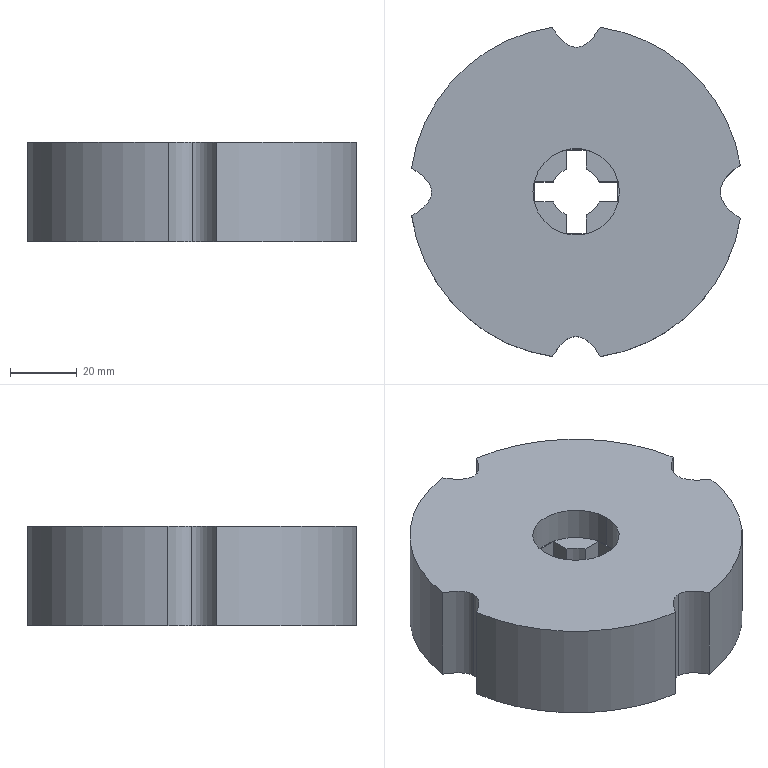Part | SolidWorks | features Extrusion 1, ICE 1 | 1 solid | 33 faces | box 98.826 x 98.952 x 30 mm | volume 216398 mm3 | plane 15 | cylinder 10 | spline 8 | commonest cylinder face diameters 15 x4 100 x4 26 x2
STEP:
#1=CARTESIAN_POINT('',(-13.,0.,5.));
#2=VERTEX_POINT('',#1);
#3=CARTESIAN_POINT('',(13.,0.,5.));
#4=VERTEX_POINT('',#3);
#5=CARTESIAN_POINT('',(0.,0.,5.));
#6=DIRECTION('',(0.,0.,1.));
#7=DIRECTION('',(1.,0.,0.));
#8=AXIS2_PLACEMENT_3D('',#5,#6,#7);
#9=CIRCLE('',#8,13.);
#10=EDGE_CURVE('',#2,#4,#9,.T.);
#11=ORIENTED_EDGE('',*,*,#10,.F.);
#12=CARTESIAN_POINT('',(-13.,0.,15.));
#13=VERTEX_POINT('',#12);
#14=CARTESIAN_POINT('',(-13.,0.,5.));
#15=DIRECTION('',(0.,0.,1.));
#16=VECTOR('',#15,1000.);
#17=LINE('',#14,#16);
#18=EDGE_CURVE('',#2,#13,#17,.T.);
#19=ORIENTED_EDGE('',*,*,#18,.T.);
#20=CARTESIAN_POINT('',(13.,0.,15.));
#21=VERTEX_POINT('',#20);
#22=CARTESIAN_POINT('',(0.,0.,15.));
#23=DIRECTION('',(0.,0.,1.));
#24=DIRECTION('',(1.,0.,0.));
#25=AXIS2_PLACEMENT_3D('',#22,#23,#24);
#26=CIRCLE('',#25,13.);
#27=EDGE_CURVE('',#13,#21,#26,.T.);
#28=ORIENTED_EDGE('',*,*,#27,.T.);
#29=CARTESIAN_POINT('',(13.,0.,5.));
#30=DIRECTION('',(0.,0.,1.));
#31=VECTOR('',#30,1000.);
#32=LINE('',#29,#31);
#33=EDGE_CURVE('',#4,#21,#32,.T.);
#34=ORIENTED_EDGE('',*,*,#33,.F.);
#35=EDGE_LOOP('',(#11,#19,#28,#34));
#36=FACE_OUTER_BOUND('',#35,.T.);
#37=CARTESIAN_POINT('',(0.,0.,5.));
#38=DIRECTION('',(0.,0.,1.));
#39=DIRECTION('',(1.,0.,0.));
#40=AXIS2_PLACEMENT_3D('',#37,#38,#39);
#41=CYLINDRICAL_SURFACE('',#40,13.);
#42=ADVANCED_FACE('',(#36),#41,.F.);
#43=CARTESIAN_POINT('',(43.351,0.,15.));
#44=VERTEX_POINT('',#43);
#45=CARTESIAN_POINT('',(49.351,8.032,15.));
#46=VERTEX_POINT('',#45);
#47=CARTESIAN_POINT('',(43.351,0.,15.));
#48=CARTESIAN_POINT('',(43.351,2.843,15.));
#49=CARTESIAN_POINT('',(45.399,5.586,15.));
#50=CARTESIAN_POINT('',(49.351,8.032,15.));
#51=(BOUNDED_CURVE()B_SPLINE_CURVE(3,(#47,#48,#49,#50),.UNSPECIFIED.,.F.,.F.)B_SPLINE_CURVE_WITH_KNOTS((4,4),(0.,0.5348),.UNSPECIFIED.)CURVE()GEOMETRIC_REPRESENTATION_ITEM()RATIONAL_B_SPLINE_CURVE((1.,0.9763,0.9763,1.))REPRESENTATION_ITEM(''));
#52=EDGE_CURVE('',#44,#46,#51,.T.);
#53=ORIENTED_EDGE('',*,*,#52,.F.);
#54=CARTESIAN_POINT('',(43.351,0.,-15.));
#55=VERTEX_POINT('',#54);
#56=CARTESIAN_POINT('',(43.351,0.,15.));
#57=DIRECTION('',(0.,0.,-1.));
#58=VECTOR('',#57,1000.);
#59=LINE('',#56,#58);
#60=EDGE_CURVE('',#44,#55,#59,.T.);
#61=ORIENTED_EDGE('',*,*,#60,.T.);
#62=CARTESIAN_POINT('',(49.351,8.032,-15.));
#63=VERTEX_POINT('',#62);
#64=CARTESIAN_POINT('',(43.351,0.,-15.));
#65=CARTESIAN_POINT('',(43.351,2.843,-15.));
#66=CARTESIAN_POINT('',(45.399,5.586,-15.));
#67=CARTESIAN_POINT('',(49.351,8.032,-15.));
#68=(BOUNDED_CURVE()B_SPLINE_CURVE(3,(#64,#65,#66,#67),.UNSPECIFIED.,.F.,.F.)B_SPLINE_CURVE_WITH_KNOTS((4,4),(0.,0.5348),.UNSPECIFIED.)CURVE()GEOMETRIC_REPRESENTATION_ITEM()RATIONAL_B_SPLINE_CURVE((1.,0.9763,0.9763,1.))REPRESENTATION_ITEM(''));
#69=EDGE_CURVE('',#55,#63,#68,.T.);
#70=ORIENTED_EDGE('',*,*,#69,.T.);
#71=CARTESIAN_POINT('',(49.351,8.032,15.));
#72=DIRECTION('',(0.,0.,-1.));
#73=VECTOR('',#72,1000.);
#74=LINE('',#71,#73);
#75=EDGE_CURVE('',#46,#63,#74,.T.);
#76=ORIENTED_EDGE('',*,*,#75,.F.);
#77=EDGE_LOOP('',(#53,#61,#70,#76));
#78=FACE_OUTER_BOUND('',#77,.T.);
#79=CARTESIAN_POINT('',(43.351,0.,15.));
#80=CARTESIAN_POINT('',(43.351,0.,-15.));
#81=CARTESIAN_POINT('',(43.351,2.843,15.));
#82=CARTESIAN_POINT('',(43.351,2.843,-15.));
#83=CARTESIAN_POINT('',(45.399,5.586,15.));
#84=CARTESIAN_POINT('',(45.399,5.586,-15.));
#85=CARTESIAN_POINT('',(49.351,8.032,15.));
#86=CARTESIAN_POINT('',(49.351,8.032,-15.));
#87=(BOUNDED_SURFACE()B_SPLINE_SURFACE(3,1,((#79,#80),(#81,#82),(#83,#84),(#85,#86)),.UNSPECIFIED.,.F.,.F.,.F.)B_SPLINE_SURFACE_WITH_KNOTS((4,4),(2,2),(0.,1.),(0.,1.),.UNSPECIFIED.)GEOMETRIC_REPRESENTATION_ITEM()RATIONAL_B_SPLINE_SURFACE(((1.,1.),(0.9763,0.9763),(0.9763,0.9763),(1.,1.)))REPRESENTATION_ITEM('')SURFACE());
#88=ADVANCED_FACE('',(#78),#87,.F.);
#89=CARTESIAN_POINT('',(0.,-43.476,15.));
#90=VERTEX_POINT('',#89);
#91=CARTESIAN_POINT('',(7.221,-49.476,15.));
#92=VERTEX_POINT('',#91);
#93=CARTESIAN_POINT('',(0.,-43.476,15.));
#94=CARTESIAN_POINT('',(2.524,-43.476,15.));
#95=CARTESIAN_POINT('',(4.977,-45.514,15.));
#96=CARTESIAN_POINT('',(7.221,-49.476,15.));
#97=(BOUNDED_CURVE()B_SPLINE_CURVE(3,(#93,#94,#95,#96),.UNSPECIFIED.,.F.,.F.)B_SPLINE_CURVE_WITH_KNOTS((4,4),(0.,0.4759),.UNSPECIFIED.)CURVE()GEOMETRIC_REPRESENTATION_ITEM()RATIONAL_B_SPLINE_CURVE((1.,0.9812,0.9812,1.))REPRESENTATION_ITEM(''));
#98=EDGE_CURVE('',#90,#92,#97,.T.);
#99=ORIENTED_EDGE('',*,*,#98,.F.);
#100=CARTESIAN_POINT('',(0.,-43.476,-15.));
#101=VERTEX_POINT('',#100);
#102=CARTESIAN_POINT('',(0.,-43.476,15.));
#103=DIRECTION('',(0.,0.,-1.));
#104=VECTOR('',#103,1000.);
#105=LINE('',#102,#104);
#106=EDGE_CURVE('',#90,#101,#105,.T.);
#107=ORIENTED_EDGE('',*,*,#106,.T.);
#108=CARTESIAN_POINT('',(7.221,-49.476,-15.));
#109=VERTEX_POINT('',#108);
#110=CARTESIAN_POINT('',(0.,-43.476,-15.));
#111=CARTESIAN_POINT('',(2.524,-43.476,-15.));
#112=CARTESIAN_POINT('',(4.977,-45.514,-15.));
#113=CARTESIAN_POINT('',(7.221,-49.476,-15.));
#114=(BOUNDED_CURVE()B_SPLINE_CURVE(3,(#110,#111,#112,#113),.UNSPECIFIED.,.F.,.F.)B_SPLINE_CURVE_WITH_KNOTS((4,4),(0.,0.4759),.UNSPECIFIED.)CURVE()GEOMETRIC_REPRESENTATION_ITEM()RATIONAL_B_SPLINE_CURVE((1.,0.9812,0.9812,1.))REPRESENTATION_ITEM(''));
#115=EDGE_CURVE('',#101,#109,#114,.T.);
#116=ORIENTED_EDGE('',*,*,#115,.T.);
#117=CARTESIAN_POINT('',(7.221,-49.476,15.));
#118=DIRECTION('',(0.,0.,-1.));
#119=VECTOR('',#118,1000.);
#120=LINE('',#117,#119);
#121=EDGE_CURVE('',#92,#109,#120,.T.);
#122=ORIENTED_EDGE('',*,*,#121,.F.);
#123=EDGE_LOOP('',(#99,#107,#116,#122));
#124=FACE_OUTER_BOUND('',#123,.T.);
#125=CARTESIAN_POINT('',(0.,-43.476,15.));
#126=CARTESIAN_POINT('',(0.,-43.476,-15.));
#127=CARTESIAN_POINT('',(2.524,-43.476,15.));
#128=CARTESIAN_POINT('',(2.524,-43.476,-15.));
#129=CARTESIAN_POINT('',(4.977,-45.514,15.));
#130=CARTESIAN_POINT('',(4.977,-45.514,-15.));
#131=CARTESIAN_POINT('',(7.221,-49.476,15.));
#132=CARTESIAN_POINT('',(7.221,-49.476,-15.));
#133=(BOUNDED_SURFACE()B_SPLINE_SURFACE(3,1,((#125,#126),(#127,#128),(#129,#130),(#131,#132)),.UNSPECIFIED.,.F.,.F.,.T.)B_SPLINE_SURFACE_WITH_KNOTS((4,4),(2,2),(0.,1.),(0.,1.),.UNSPECIFIED.)GEOMETRIC_REPRESENTATION_ITEM()RATIONAL_B_SPLINE_SURFACE(((1.,1.),(0.9812,0.9812),(0.9812,0.9812),(1.,1.)))REPRESENTATION_ITEM('')SURFACE());
#134=ADVANCED_FACE('',(#124),#133,.F.);
#135=CARTESIAN_POINT('',(-43.476,0.,15.));
#136=VERTEX_POINT('',#135);
#137=CARTESIAN_POINT('',(-49.476,-7.221,15.));
#138=VERTEX_POINT('',#137);
#139=CARTESIAN_POINT('',(-43.476,0.,15.));
#140=CARTESIAN_POINT('',(-43.476,-2.524,15.));
#141=CARTESIAN_POINT('',(-45.514,-4.977,15.));
#142=CARTESIAN_POINT('',(-49.476,-7.221,15.));
#143=(BOUNDED_CURVE()B_SPLINE_CURVE(3,(#139,#140,#141,#142),.UNSPECIFIED.,.F.,.F.)B_SPLINE_CURVE_WITH_KNOTS((4,4),(0.,0.4759),.UNSPECIFIED.)CURVE()GEOMETRIC_REPRESENTATION_ITEM()RATIONAL_B_SPLINE_CURVE((1.,0.9812,0.9812,1.))REPRESENTATION_ITEM(''));
#144=EDGE_CURVE('',#136,#138,#143,.T.);
#145=ORIENTED_EDGE('',*,*,#144,.F.);
#146=CARTESIAN_POINT('',(-43.476,0.,-15.));
#147=VERTEX_POINT('',#146);
#148=CARTESIAN_POINT('',(-43.476,0.,15.));
#149=DIRECTION('',(0.,0.,-1.));
#150=VECTOR('',#149,1000.);
#151=LINE('',#148,#150);
#152=EDGE_CURVE('',#136,#147,#151,.T.);
#153=ORIENTED_EDGE('',*,*,#152,.T.);
#154=CARTESIAN_POINT('',(-49.476,-7.221,-15.));
#155=VERTEX_POINT('',#154);
#156=CARTESIAN_POINT('',(-43.476,0.,-15.));
#157=CARTESIAN_POINT('',(-43.476,-2.524,-15.));
#158=CARTESIAN_POINT('',(-45.514,-4.977,-15.));
#159=CARTESIAN_POINT('',(-49.476,-7.221,-15.));
#160=(BOUNDED_CURVE()B_SPLINE_CURVE(3,(#156,#157,#158,#159),.UNSPECIFIED.,.F.,.T.)B_SPLINE_CURVE_WITH_KNOTS((4,4),(0.,0.4759),.UNSPECIFIED.)CURVE()GEOMETRIC_REPRESENTATION_ITEM()RATIONAL_B_SPLINE_CURVE((1.,0.9812,0.9812,1.))REPRESENTATION_ITEM(''));
#161=EDGE_CURVE('',#147,#155,#160,.T.);
#162=ORIENTED_EDGE('',*,*,#161,.T.);
#163=CARTESIAN_POINT('',(-49.476,-7.221,15.));
#164=DIRECTION('',(0.,0.,-1.));
#165=VECTOR('',#164,1000.);
#166=LINE('',#163,#165);
#167=EDGE_CURVE('',#138,#155,#166,.T.);
#168=ORIENTED_EDGE('',*,*,#167,.F.);
#169=EDGE_LOOP('',(#145,#153,#162,#168));
#170=FACE_OUTER_BOUND('',#169,.T.);
#171=CARTESIAN_POINT('',(-43.476,0.,15.));
#172=CARTESIAN_POINT('',(-43.476,0.,-15.));
#173=CARTESIAN_POINT('',(-43.476,-2.524,15.));
#174=CARTESIAN_POINT('',(-43.476,-2.524,-15.));
#175=CARTESIAN_POINT('',(-45.514,-4.977,15.));
#176=CARTESIAN_POINT('',(-45.514,-4.977,-15.));
#177=CARTESIAN_POINT('',(-49.476,-7.221,15.));
#178=CARTESIAN_POINT('',(-49.476,-7.221,-15.));
#179=(BOUNDED_SURFACE()B_SPLINE_SURFACE(3,1,((#171,#172),(#173,#174),(#175,#176),(#177,#178)),.UNSPECIFIED.,.F.,.F.,.T.)B_SPLINE_SURFACE_WITH_KNOTS((4,4),(2,2),(0.,1.),(0.,1.),.UNSPECIFIED.)GEOMETRIC_REPRESENTATION_ITEM()RATIONAL_B_SPLINE_SURFACE(((1.,1.),(0.9812,0.9812),(0.9812,0.9812),(1.,1.)))REPRESENTATION_ITEM('')SURFACE());
#180=ADVANCED_FACE('',(#170),#179,.F.);
#181=CARTESIAN_POINT('',(0.,43.476,15.));
#182=VERTEX_POINT('',#181);
#183=CARTESIAN_POINT('',(-7.221,49.476,15.));
#184=VERTEX_POINT('',#183);
#185=CARTESIAN_POINT('',(0.,43.476,15.));
#186=CARTESIAN_POINT('',(-2.524,43.476,15.));
#187=CARTESIAN_POINT('',(-4.977,45.514,15.));
#188=CARTESIAN_POINT('',(-7.221,49.476,15.));
#189=(BOUNDED_CURVE()B_SPLINE_CURVE(3,(#185,#186,#187,#188),.UNSPECIFIED.,.F.,.F.)B_SPLINE_CURVE_WITH_KNOTS((4,4),(0.,0.4759),.UNSPECIFIED.)CURVE()GEOMETRIC_REPRESENTATION_ITEM()RATIONAL_B_SPLINE_CURVE((1.,0.9812,0.9812,1.))REPRESENTATION_ITEM(''));
#190=EDGE_CURVE('',#182,#184,#189,.T.);
#191=ORIENTED_EDGE('',*,*,#190,.F.);
#192=CARTESIAN_POINT('',(0.,43.476,-15.));
#193=VERTEX_POINT('',#192);
#194=CARTESIAN_POINT('',(0.,43.476,15.));
#195=DIRECTION('',(0.,0.,-1.));
#196=VECTOR('',#195,1000.);
#197=LINE('',#194,#196);
#198=EDGE_CURVE('',#182,#193,#197,.T.);
#199=ORIENTED_EDGE('',*,*,#198,.T.);
#200=CARTESIAN_POINT('',(-7.221,49.476,-15.));
#201=VERTEX_POINT('',#200);
#202=CARTESIAN_POINT('',(0.,43.476,-15.));
#203=CARTESIAN_POINT('',(-2.524,43.476,-15.));
#204=CARTESIAN_POINT('',(-4.977,45.514,-15.));
#205=CARTESIAN_POINT('',(-7.221,49.476,-15.));
#206=(BOUNDED_CURVE()B_SPLINE_CURVE(3,(#202,#203,#204,#205),.UNSPECIFIED.,.F.,.F.)B_SPLINE_CURVE_WITH_KNOTS((4,4),(0.,0.4759),.UNSPECIFIED.)CURVE()GEOMETRIC_REPRESENTATION_ITEM()RATIONAL_B_SPLINE_CURVE((1.,0.9812,0.9812,1.))REPRESENTATION_ITEM(''));
#207=EDGE_CURVE('',#193,#201,#206,.T.);
#208=ORIENTED_EDGE('',*,*,#207,.T.);
#209=CARTESIAN_POINT('',(-7.221,49.476,15.));
#210=DIRECTION('',(0.,0.,-1.));
#211=VECTOR('',#210,1000.);
#212=LINE('',#209,#211);
#213=EDGE_CURVE('',#184,#201,#212,.T.);
#214=ORIENTED_EDGE('',*,*,#213,.F.);
#215=EDGE_LOOP('',(#191,#199,#208,#214));
#216=FACE_OUTER_BOUND('',#215,.T.);
#217=CARTESIAN_POINT('',(0.,43.476,15.));
#218=CARTESIAN_POINT('',(0.,43.476,-15.));
#219=CARTESIAN_POINT('',(-2.524,43.476,15.));
#220=CARTESIAN_POINT('',(-2.524,43.476,-15.));
#221=CARTESIAN_POINT('',(-4.977,45.514,15.));
#222=CARTESIAN_POINT('',(-4.977,45.514,-15.));
#223=CARTESIAN_POINT('',(-7.221,49.476,15.));
#224=CARTESIAN_POINT('',(-7.221,49.476,-15.));
#225=(BOUNDED_SURFACE()B_SPLINE_SURFACE(3,1,((#217,#218),(#219,#220),(#221,#222),(#223,#224)),.UNSPECIFIED.,.F.,.F.,.T.)B_SPLINE_SURFACE_WITH_KNOTS((4,4),(2,2),(0.,1.),(0.,1.),.UNSPECIFIED.)GEOMETRIC_REPRESENTATION_ITEM()RATIONAL_B_SPLINE_SURFACE(((1.,1.),(0.9812,0.9812),(0.9812,0.9812),(1.,1.)))REPRESENTATION_ITEM('')SURFACE());
#226=ADVANCED_FACE('',(#216),#225,.F.);
#227=CARTESIAN_POINT('',(6.874,3.,5.));
#228=VERTEX_POINT('',#227);
#229=CARTESIAN_POINT('',(6.874,3.,-15.));
#230=VERTEX_POINT('',#229);
#231=CARTESIAN_POINT('',(6.874,3.,15.));
#232=DIRECTION('',(0.,0.,-1.));
#233=VECTOR('',#232,1000.);
#234=LINE('',#231,#233);
#235=EDGE_CURVE('',#228,#230,#234,.T.);
#236=ORIENTED_EDGE('',*,*,#235,.F.);
#237=CARTESIAN_POINT('',(3.,6.874,5.));
#238=VERTEX_POINT('',#237);
#239=CARTESIAN_POINT('',(0.,0.,5.));
#240=DIRECTION('',(0.,0.,1.));
#241=DIRECTION('',(1.,0.,0.));
#242=AXIS2_PLACEMENT_3D('',#239,#240,#241);
#243=CIRCLE('',#242,7.5);
#244=EDGE_CURVE('',#228,#238,#243,.T.);
#245=ORIENTED_EDGE('',*,*,#244,.T.);
#246=CARTESIAN_POINT('',(3.,6.874,-15.));
#247=VERTEX_POINT('',#246);
#248=CARTESIAN_POINT('',(3.,6.874,15.));
#249=DIRECTION('',(0.,0.,-1.));
#250=VECTOR('',#249,1000.);
#251=LINE('',#248,#250);
#252=EDGE_CURVE('',#238,#247,#251,.T.);
#253=ORIENTED_EDGE('',*,*,#252,.T.);
#254=CARTESIAN_POINT('',(0.,0.,-15.));
#255=DIRECTION('',(0.,0.,1.));
#256=DIRECTION('',(1.,0.,0.));
#257=AXIS2_PLACEMENT_3D('',#254,#255,#256);
#258=CIRCLE('',#257,7.5);
#259=EDGE_CURVE('',#230,#247,#258,.T.);
#260=ORIENTED_EDGE('',*,*,#259,.F.);
#261=EDGE_LOOP('',(#236,#245,#253,#260));
#262=FACE_OUTER_BOUND('',#261,.T.);
#263=CARTESIAN_POINT('',(0.,0.,15.));
#264=DIRECTION('',(0.,0.,-1.));
#265=DIRECTION('',(-1.,0.,0.));
#266=AXIS2_PLACEMENT_3D('',#263,#264,#265);
#267=CYLINDRICAL_SURFACE('',#266,7.5);
#268=ADVANCED_FACE('',(#262),#267,.F.);
#269=ORIENTED_EDGE('',*,*,#252,.F.);
#270=CARTESIAN_POINT('',(3.,12.5,5.));
#271=VERTEX_POINT('',#270);
#272=CARTESIAN_POINT('',(3.,12.5,5.));
#273=DIRECTION('',(0.,1.,0.));
#274=VECTOR('',#273,1000.);
#275=LINE('',#272,#274);
#276=EDGE_CURVE('',#238,#271,#275,.T.);
#277=ORIENTED_EDGE('',*,*,#276,.T.);
#278=CARTESIAN_POINT('',(3.,12.5,-15.));
#279=VERTEX_POINT('',#278);
#280=CARTESIAN_POINT('',(3.,12.5,15.));
#281=DIRECTION('',(0.,0.,-1.));
#282=VECTOR('',#281,1000.);
#283=LINE('',#280,#282);
#284=EDGE_CURVE('',#271,#279,#283,.T.);
#285=ORIENTED_EDGE('',*,*,#284,.T.);
#286=CARTESIAN_POINT('',(3.,12.5,-15.));
#287=DIRECTION('',(0.,1.,0.));
#288=VECTOR('',#287,1000.);
#289=LINE('',#286,#288);
#290=EDGE_CURVE('',#247,#279,#289,.T.);
#291=ORIENTED_EDGE('',*,*,#290,.F.);
#292=EDGE_LOOP('',(#269,#277,#285,#291));
#293=FACE_OUTER_BOUND('',#292,.T.);
#294=CARTESIAN_POINT('',(3.,12.5,15.));
#295=DIRECTION('',(-1.,0.,0.));
#296=DIRECTION('',(0.,-1.,0.));
#297=AXIS2_PLACEMENT_3D('',#294,#295,#296);
#298=PLANE('',#297);
#299=ADVANCED_FACE('',(#293),#298,.T.);
#300=ORIENTED_EDGE('',*,*,#284,.F.);
#301=CARTESIAN_POINT('',(-3.,12.5,5.));
#302=VERTEX_POINT('',#301);
#303=CARTESIAN_POINT('',(-3.,12.5,5.));
#304=DIRECTION('',(-1.,0.,0.));
#305=VECTOR('',#304,1000.);
#306=LINE('',#303,#305);
#307=EDGE_CURVE('',#271,#302,#306,.T.);
#308=ORIENTED_EDGE('',*,*,#307,.T.);
#309=CARTESIAN_POINT('',(-3.,12.5,-15.));
#310=VERTEX_POINT('',#309);
#311=CARTESIAN_POINT('',(-3.,12.5,15.));
#312=DIRECTION('',(0.,0.,-1.));
#313=VECTOR('',#312,1000.);
#314=LINE('',#311,#313);
#315=EDGE_CURVE('',#302,#310,#314,.T.);
#316=ORIENTED_EDGE('',*,*,#315,.T.);
#317=CARTESIAN_POINT('',(-3.,12.5,-15.));
#318=DIRECTION('',(-1.,0.,0.));
#319=VECTOR('',#318,1000.);
#320=LINE('',#317,#319);
#321=EDGE_CURVE('',#279,#310,#320,.T.);
#322=ORIENTED_EDGE('',*,*,#321,.F.);
#323=EDGE_LOOP('',(#300,#308,#316,#322));
#324=FACE_OUTER_BOUND('',#323,.T.);
#325=CARTESIAN_POINT('',(-3.,12.5,15.));
#326=DIRECTION('',(0.,-1.,0.));
#327=DIRECTION('',(0.,0.,-1.));
#328=AXIS2_PLACEMENT_3D('',#325,#326,#327);
#329=PLANE('',#328);
#330=ADVANCED_FACE('',(#324),#329,.T.);
#331=ORIENTED_EDGE('',*,*,#315,.F.);
#332=CARTESIAN_POINT('',(-3.,6.874,5.));
#333=VERTEX_POINT('',#332);
#334=CARTESIAN_POINT('',(-3.,12.5,5.));
#335=DIRECTION('',(0.,-1.,0.));
#336=VECTOR('',#335,1000.);
#337=LINE('',#334,#336);
#338=EDGE_CURVE('',#302,#333,#337,.T.);
#339=ORIENTED_EDGE('',*,*,#338,.T.);
#340=CARTESIAN_POINT('',(-3.,6.874,-15.));
#341=VERTEX_POINT('',#340);
#342=CARTESIAN_POINT('',(-3.,6.874,15.));
#343=DIRECTION('',(0.,0.,-1.));
#344=VECTOR('',#343,1000.);
#345=LINE('',#342,#344);
#346=EDGE_CURVE('',#333,#341,#345,.T.);
#347=ORIENTED_EDGE('',*,*,#346,.T.);
#348=CARTESIAN_POINT('',(-3.,12.5,-15.));
#349=DIRECTION('',(0.,-1.,0.));
#350=VECTOR('',#349,1000.);
#351=LINE('',#348,#350);
#352=EDGE_CURVE('',#310,#341,#351,.T.);
#353=ORIENTED_EDGE('',*,*,#352,.F.);
#354=EDGE_LOOP('',(#331,#339,#347,#353));
#355=FACE_OUTER_BOUND('',#354,.T.);
#356=CARTESIAN_POINT('',(-3.,12.5,15.));
#357=DIRECTION('',(1.,0.,0.));
#358=DIRECTION('',(0.,1.,0.));
#359=AXIS2_PLACEMENT_3D('',#356,#357,#358);
#360=PLANE('',#359);
#361=ADVANCED_FACE('',(#355),#360,.T.);
#362=ORIENTED_EDGE('',*,*,#346,.F.);
#363=CARTESIAN_POINT('',(-6.874,3.,5.));
#364=VERTEX_POINT('',#363);
#365=CARTESIAN_POINT('',(0.,0.,5.));
#366=DIRECTION('',(0.,0.,1.));
#367=DIRECTION('',(1.,0.,0.));
#368=AXIS2_PLACEMENT_3D('',#365,#366,#367);
#369=CIRCLE('',#368,7.5);
#370=EDGE_CURVE('',#333,#364,#369,.T.);
#371=ORIENTED_EDGE('',*,*,#370,.T.);
#372=CARTESIAN_POINT('',(-6.874,3.,-15.));
#373=VERTEX_POINT('',#372);
#374=CARTESIAN_POINT('',(-6.874,3.,15.));
#375=DIRECTION('',(0.,0.,-1.));
#376=VECTOR('',#375,1000.);
#377=LINE('',#374,#376);
#378=EDGE_CURVE('',#364,#373,#377,.T.);
#379=ORIENTED_EDGE('',*,*,#378,.T.);
#380=CARTESIAN_POINT('',(0.,0.,-15.));
#381=DIRECTION('',(0.,0.,1.));
#382=DIRECTION('',(1.,0.,0.));
#383=AXIS2_PLACEMENT_3D('',#380,#381,#382);
#384=CIRCLE('',#383,7.5);
#385=EDGE_CURVE('',#341,#373,#384,.T.);
#386=ORIENTED_EDGE('',*,*,#385,.F.);
#387=EDGE_LOOP('',(#362,#371,#379,#386));
#388=FACE_OUTER_BOUND('',#387,.T.);
#389=CARTESIAN_POINT('',(0.,0.,15.));
#390=DIRECTION('',(0.,0.,-1.));
#391=DIRECTION('',(-1.,0.,0.));
#392=AXIS2_PLACEMENT_3D('',#389,#390,#391);
#393=CYLINDRICAL_SURFACE('',#392,7.5);
#394=ADVANCED_FACE('',(#388),#393,.F.);
#395=ORIENTED_EDGE('',*,*,#378,.F.);
#396=CARTESIAN_POINT('',(-12.5,3.,5.));
#397=VERTEX_POINT('',#396);
#398=CARTESIAN_POINT('',(-12.5,3.,5.));
#399=DIRECTION('',(-1.,0.,0.));
#400=VECTOR('',#399,1000.);
#401=LINE('',#398,#400);
#402=EDGE_CURVE('',#364,#397,#401,.T.);
#403=ORIENTED_EDGE('',*,*,#402,.T.);
#404=CARTESIAN_POINT('',(-12.5,3.,-15.));
#405=VERTEX_POINT('',#404);
#406=CARTESIAN_POINT('',(-12.5,3.,15.));
#407=DIRECTION('',(0.,0.,-1.));
#408=VECTOR('',#407,1000.);
#409=LINE('',#406,#408);
#410=EDGE_CURVE('',#397,#405,#409,.T.);
#411=ORIENTED_EDGE('',*,*,#410,.T.);
#412=CARTESIAN_POINT('',(-12.5,3.,-15.));
#413=DIRECTION('',(-1.,0.,0.));
#414=VECTOR('',#413,1000.);
#415=LINE('',#412,#414);
#416=EDGE_CURVE('',#373,#405,#415,.T.);
#417=ORIENTED_EDGE('',*,*,#416,.F.);
#418=EDGE_LOOP('',(#395,#403,#411,#417));
#419=FACE_OUTER_BOUND('',#418,.T.);
#420=CARTESIAN_POINT('',(-12.5,3.,15.));
#421=DIRECTION('',(0.,-1.,0.));
#422=DIRECTION('',(0.,0.,-1.));
#423=AXIS2_PLACEMENT_3D('',#420,#421,#422);
#424=PLANE('',#423);
#425=ADVANCED_FACE('',(#419),#424,.T.);
#426=ORIENTED_EDGE('',*,*,#410,.F.);
#427=CARTESIAN_POINT('',(-12.5,-3.,5.));
#428=VERTEX_POINT('',#427);
#429=CARTESIAN_POINT('',(-12.5,-3.,5.));
#430=DIRECTION('',(0.,-1.,0.));
#431=VECTOR('',#430,1000.);
#432=LINE('',#429,#431);
#433=EDGE_CURVE('',#397,#428,#432,.T.);
#434=ORIENTED_EDGE('',*,*,#433,.T.);
#435=CARTESIAN_POINT('',(-12.5,-3.,-15.));
#436=VERTEX_POINT('',#435);
#437=CARTESIAN_POINT('',(-12.5,-3.,15.));
#438=DIRECTION('',(0.,0.,-1.));
#439=VECTOR('',#438,1000.);
#440=LINE('',#437,#439);
#441=EDGE_CURVE('',#428,#436,#440,.T.);
#442=ORIENTED_EDGE('',*,*,#441,.T.);
#443=CARTESIAN_POINT('',(-12.5,-3.,-15.));
#444=DIRECTION('',(0.,-1.,0.));
#445=VECTOR('',#444,1000.);
#446=LINE('',#443,#445);
#447=EDGE_CURVE('',#405,#436,#446,.T.);
#448=ORIENTED_EDGE('',*,*,#447,.F.);
#449=EDGE_LOOP('',(#426,#434,#442,#448));
#450=FACE_OUTER_BOUND('',#449,.T.);
#451=CARTESIAN_POINT('',(-12.5,-3.,15.));
#452=DIRECTION('',(1.,0.,0.));
#453=DIRECTION('',(0.,1.,0.));
#454=AXIS2_PLACEMENT_3D('',#451,#452,#453);
#455=PLANE('',#454);
#456=ADVANCED_FACE('',(#450),#455,.T.);
#457=ORIENTED_EDGE('',*,*,#441,.F.);
#458=CARTESIAN_POINT('',(-6.874,-3.,5.));
#459=VERTEX_POINT('',#458);
#460=CARTESIAN_POINT('',(-12.5,-3.,5.));
#461=DIRECTION('',(1.,0.,0.));
#462=VECTOR('',#461,1000.);
#463=LINE('',#460,#462);
#464=EDGE_CURVE('',#428,#459,#463,.T.);
#465=ORIENTED_EDGE('',*,*,#464,.T.);
#466=CARTESIAN_POINT('',(-6.874,-3.,-15.));
#467=VERTEX_POINT('',#466);
#468=CARTESIAN_POINT('',(-6.874,-3.,15.));
#469=DIRECTION('',(0.,0.,-1.));
#470=VECTOR('',#469,1000.);
#471=LINE('',#468,#470);
#472=EDGE_CURVE('',#459,#467,#471,.T.);
#473=ORIENTED_EDGE('',*,*,#472,.T.);
#474=CARTESIAN_POINT('',(-12.5,-3.,-15.));
#475=DIRECTION('',(1.,0.,0.));
#476=VECTOR('',#475,1000.);
#477=LINE('',#474,#476);
#478=EDGE_CURVE('',#436,#467,#477,.T.);
#479=ORIENTED_EDGE('',*,*,#478,.F.);
#480=EDGE_LOOP('',(#457,#465,#473,#479));
#481=FACE_OUTER_BOUND('',#480,.T.);
#482=CARTESIAN_POINT('',(-12.5,-3.,15.));
#483=DIRECTION('',(0.,1.,0.));
#484=DIRECTION('',(-1.,0.,0.));
#485=AXIS2_PLACEMENT_3D('',#482,#483,#484);
#486=PLANE('',#485);
#487=ADVANCED_FACE('',(#481),#486,.T.);
#488=ORIENTED_EDGE('',*,*,#472,.F.);
#489=CARTESIAN_POINT('',(-3.,-6.874,5.));
#490=VERTEX_POINT('',#489);
#491=CARTESIAN_POINT('',(0.,0.,5.));
#492=DIRECTION('',(0.,0.,1.));
#493=DIRECTION('',(1.,0.,0.));
#494=AXIS2_PLACEMENT_3D('',#491,#492,#493);
#495=CIRCLE('',#494,7.5);
#496=EDGE_CURVE('',#459,#490,#495,.T.);
#497=ORIENTED_EDGE('',*,*,#496,.T.);
#498=CARTESIAN_POINT('',(-3.,-6.874,-15.));
#499=VERTEX_POINT('',#498);
#500=CARTESIAN_POINT('',(-3.,-6.874,15.));
#501=DIRECTION('',(0.,0.,-1.));
#502=VECTOR('',#501,1000.);
#503=LINE('',#500,#502);
#504=EDGE_CURVE('',#490,#499,#503,.T.);
#505=ORIENTED_EDGE('',*,*,#504,.T.);
#506=CARTESIAN_POINT('',(0.,0.,-15.));
#507=DIRECTION('',(0.,0.,1.));
#508=DIRECTION('',(1.,0.,0.));
#509=AXIS2_PLACEMENT_3D('',#506,#507,#508);
#510=CIRCLE('',#509,7.5);
#511=EDGE_CURVE('',#467,#499,#510,.T.);
#512=ORIENTED_EDGE('',*,*,#511,.F.);
#513=EDGE_LOOP('',(#488,#497,#505,#512));
#514=FACE_OUTER_BOUND('',#513,.T.);
#515=CARTESIAN_POINT('',(0.,0.,15.));
#516=DIRECTION('',(0.,0.,-1.));
#517=DIRECTION('',(-1.,0.,0.));
#518=AXIS2_PLACEMENT_3D('',#515,#516,#517);
#519=CYLINDRICAL_SURFACE('',#518,7.5);
#520=ADVANCED_FACE('',(#514),#519,.F.);
#521=ORIENTED_EDGE('',*,*,#504,.F.);
#522=CARTESIAN_POINT('',(-3.,-12.5,5.));
#523=VERTEX_POINT('',#522);
#524=CARTESIAN_POINT('',(-3.,-6.874,5.));
#525=DIRECTION('',(0.,-1.,0.));
#526=VECTOR('',#525,1000.);
#527=LINE('',#524,#526);
#528=EDGE_CURVE('',#490,#523,#527,.T.);
#529=ORIENTED_EDGE('',*,*,#528,.T.);
#530=CARTESIAN_POINT('',(-3.,-12.5,-15.));
#531=VERTEX_POINT('',#530);
#532=CARTESIAN_POINT('',(-3.,-12.5,15.));
#533=DIRECTION('',(0.,0.,-1.));
#534=VECTOR('',#533,1000.);
#535=LINE('',#532,#534);
#536=EDGE_CURVE('',#523,#531,#535,.T.);
#537=ORIENTED_EDGE('',*,*,#536,.T.);
#538=CARTESIAN_POINT('',(-3.,-6.874,-15.));
#539=DIRECTION('',(0.,-1.,0.));
#540=VECTOR('',#539,1000.);
#541=LINE('',#538,#540);
#542=EDGE_CURVE('',#499,#531,#541,.T.);
#543=ORIENTED_EDGE('',*,*,#542,.F.);
#544=EDGE_LOOP('',(#521,#529,#537,#543));
#545=FACE_OUTER_BOUND('',#544,.T.);
#546=CARTESIAN_POINT('',(-3.,-6.874,15.));
#547=DIRECTION('',(1.,0.,0.));
#548=DIRECTION('',(0.,1.,0.));
#549=AXIS2_PLACEMENT_3D('',#546,#547,#548);
#550=PLANE('',#549);
#551=ADVANCED_FACE('',(#545),#550,.T.);
#552=ORIENTED_EDGE('',*,*,#536,.F.);
#553=CARTESIAN_POINT('',(3.,-12.5,5.));
#554=VERTEX_POINT('',#553);
#555=CARTESIAN_POINT('',(-3.,-12.5,5.));
#556=DIRECTION('',(1.,0.,0.));
#557=VECTOR('',#556,1000.);
#558=LINE('',#555,#557);
#559=EDGE_CURVE('',#523,#554,#558,.T.);
#560=ORIENTED_EDGE('',*,*,#559,.T.);
#561=CARTESIAN_POINT('',(3.,-12.5,-15.));
#562=VERTEX_POINT('',#561);
#563=CARTESIAN_POINT('',(3.,-12.5,15.));
#564=DIRECTION('',(0.,0.,-1.));
#565=VECTOR('',#564,1000.);
#566=LINE('',#563,#565);
#567=EDGE_CURVE('',#554,#562,#566,.T.);
#568=ORIENTED_EDGE('',*,*,#567,.T.);
#569=CARTESIAN_POINT('',(-3.,-12.5,-15.));
#570=DIRECTION('',(1.,0.,0.));
#571=VECTOR('',#570,1000.);
#572=LINE('',#569,#571);
#573=EDGE_CURVE('',#531,#562,#572,.T.);
#574=ORIENTED_EDGE('',*,*,#573,.F.);
#575=EDGE_LOOP('',(#552,#560,#568,#574));
#576=FACE_OUTER_BOUND('',#575,.T.);
#577=CARTESIAN_POINT('',(-3.,-12.5,15.));
#578=DIRECTION('',(0.,1.,0.));
#579=DIRECTION('',(0.,0.,1.));
#580=AXIS2_PLACEMENT_3D('',#577,#578,#579);
#581=PLANE('',#580);
#582=ADVANCED_FACE('',(#576),#581,.T.);
#583=ORIENTED_EDGE('',*,*,#567,.F.);
#584=CARTESIAN_POINT('',(3.,-6.874,5.));
#585=VERTEX_POINT('',#584);
#586=CARTESIAN_POINT('',(3.,-6.874,5.));
#587=DIRECTION('',(0.,1.,0.));
#588=VECTOR('',#587,1000.);
#589=LINE('',#586,#588);
#590=EDGE_CURVE('',#554,#585,#589,.T.);
#591=ORIENTED_EDGE('',*,*,#590,.T.);
#592=CARTESIAN_POINT('',(3.,-6.874,-15.));
#593=VERTEX_POINT('',#592);
#594=CARTESIAN_POINT('',(3.,-6.874,15.));
#595=DIRECTION('',(0.,0.,-1.));
#596=VECTOR('',#595,1000.);
#597=LINE('',#594,#596);
#598=EDGE_CURVE('',#585,#593,#597,.T.);
#599=ORIENTED_EDGE('',*,*,#598,.T.);
#600=CARTESIAN_POINT('',(3.,-6.874,-15.));
#601=DIRECTION('',(0.,1.,0.));
#602=VECTOR('',#601,1000.);
#603=LINE('',#600,#602);
#604=EDGE_CURVE('',#562,#593,#603,.T.);
#605=ORIENTED_EDGE('',*,*,#604,.F.);
#606=EDGE_LOOP('',(#583,#591,#599,#605));
#607=FACE_OUTER_BOUND('',#606,.T.);
#608=CARTESIAN_POINT('',(3.,-6.874,15.));
#609=DIRECTION('',(-1.,0.,0.));
#610=DIRECTION('',(0.,-1.,0.));
#611=AXIS2_PLACEMENT_3D('',#608,#609,#610);
#612=PLANE('',#611);
#613=ADVANCED_FACE('',(#607),#612,.T.);
#614=ORIENTED_EDGE('',*,*,#598,.F.);
#615=CARTESIAN_POINT('',(6.874,-3.,5.));
#616=VERTEX_POINT('',#615);
#617=CARTESIAN_POINT('',(0.,0.,5.));
#618=DIRECTION('',(0.,0.,1.));
#619=DIRECTION('',(1.,0.,0.));
#620=AXIS2_PLACEMENT_3D('',#617,#618,#619);
#621=CIRCLE('',#620,7.5);
#622=EDGE_CURVE('',#585,#616,#621,.T.);
#623=ORIENTED_EDGE('',*,*,#622,.T.);
#624=CARTESIAN_POINT('',(6.874,-3.,-15.));
#625=VERTEX_POINT('',#624);
#626=CARTESIAN_POINT('',(6.874,-3.,15.));
#627=DIRECTION('',(0.,0.,-1.));
#628=VECTOR('',#627,1000.);
#629=LINE('',#626,#628);
#630=EDGE_CURVE('',#616,#625,#629,.T.);
#631=ORIENTED_EDGE('',*,*,#630,.T.);
#632=CARTESIAN_POINT('',(0.,0.,-15.));
#633=DIRECTION('',(0.,0.,1.));
#634=DIRECTION('',(1.,0.,0.));
#635=AXIS2_PLACEMENT_3D('',#632,#633,#634);
#636=CIRCLE('',#635,7.5);
#637=EDGE_CURVE('',#593,#625,#636,.T.);
#638=ORIENTED_EDGE('',*,*,#637,.F.);
#639=EDGE_LOOP('',(#614,#623,#631,#638));
#640=FACE_OUTER_BOUND('',#639,.T.);
#641=CARTESIAN_POINT('',(0.,0.,15.));
#642=DIRECTION('',(0.,0.,-1.));
#643=DIRECTION('',(-1.,0.,0.));
#644=AXIS2_PLACEMENT_3D('',#641,#642,#643);
#645=CYLINDRICAL_SURFACE('',#644,7.5);
#646=ADVANCED_FACE('',(#640),#645,.F.);
#647=ORIENTED_EDGE('',*,*,#630,.F.);
#648=CARTESIAN_POINT('',(12.5,-3.,5.));
#649=VERTEX_POINT('',#648);
#650=CARTESIAN_POINT('',(6.874,-3.,5.));
#651=DIRECTION('',(1.,0.,0.));
#652=VECTOR('',#651,1000.);
#653=LINE('',#650,#652);
#654=EDGE_CURVE('',#616,#649,#653,.T.);
#655=ORIENTED_EDGE('',*,*,#654,.T.);
#656=CARTESIAN_POINT('',(12.5,-3.,-15.));
#657=VERTEX_POINT('',#656);
#658=CARTESIAN_POINT('',(12.5,-3.,15.));
#659=DIRECTION('',(0.,0.,-1.));
#660=VECTOR('',#659,1000.);
#661=LINE('',#658,#660);
#662=EDGE_CURVE('',#649,#657,#661,.T.);
#663=ORIENTED_EDGE('',*,*,#662,.T.);
#664=CARTESIAN_POINT('',(6.874,-3.,-15.));
#665=DIRECTION('',(1.,0.,0.));
#666=VECTOR('',#665,1000.);
#667=LINE('',#664,#666);
#668=EDGE_CURVE('',#625,#657,#667,.T.);
#669=ORIENTED_EDGE('',*,*,#668,.F.);
#670=EDGE_LOOP('',(#647,#655,#663,#669));
#671=FACE_OUTER_BOUND('',#670,.T.);
#672=CARTESIAN_POINT('',(6.874,-3.,15.));
#673=DIRECTION('',(0.,1.,0.));
#674=DIRECTION('',(0.,0.,1.));
#675=AXIS2_PLACEMENT_3D('',#672,#673,#674);
#676=PLANE('',#675);
#677=ADVANCED_FACE('',(#671),#676,.T.);
#678=ORIENTED_EDGE('',*,*,#662,.F.);
#679=CARTESIAN_POINT('',(12.5,3.,5.));
#680=VERTEX_POINT('',#679);
#681=CARTESIAN_POINT('',(12.5,-3.,5.));
#682=DIRECTION('',(0.,1.,0.));
#683=VECTOR('',#682,1000.);
#684=LINE('',#681,#683);
#685=EDGE_CURVE('',#649,#680,#684,.T.);
#686=ORIENTED_EDGE('',*,*,#685,.T.);
#687=CARTESIAN_POINT('',(12.5,3.,-15.));
#688=VERTEX_POINT('',#687);
#689=CARTESIAN_POINT('',(12.5,3.,15.));
#690=DIRECTION('',(0.,0.,-1.));
#691=VECTOR('',#690,1000.);
#692=LINE('',#689,#691);
#693=EDGE_CURVE('',#680,#688,#692,.T.);
#694=ORIENTED_EDGE('',*,*,#693,.T.);
#695=CARTESIAN_POINT('',(12.5,-3.,-15.));
#696=DIRECTION('',(0.,1.,0.));
#697=VECTOR('',#696,1000.);
#698=LINE('',#695,#697);
#699=EDGE_CURVE('',#657,#688,#698,.T.);
#700=ORIENTED_EDGE('',*,*,#699,.F.);
#701=EDGE_LOOP('',(#678,#686,#694,#700));
#702=FACE_OUTER_BOUND('',#701,.T.);
#703=CARTESIAN_POINT('',(12.5,-3.,15.));
#704=DIRECTION('',(-1.,0.,0.));
#705=DIRECTION('',(0.,-1.,0.));
#706=AXIS2_PLACEMENT_3D('',#703,#704,#705);
#707=PLANE('',#706);
#708=ADVANCED_FACE('',(#702),#707,.T.);
#709=ORIENTED_EDGE('',*,*,#693,.F.);
#710=CARTESIAN_POINT('',(6.874,3.,5.));
#711=DIRECTION('',(-1.,0.,0.));
#712=VECTOR('',#711,1000.);
#713=LINE('',#710,#712);
#714=EDGE_CURVE('',#680,#228,#713,.T.);
#715=ORIENTED_EDGE('',*,*,#714,.T.);
#716=ORIENTED_EDGE('',*,*,#235,.T.);
#717=CARTESIAN_POINT('',(6.874,3.,-15.));
#718=DIRECTION('',(-1.,0.,0.));
#719=VECTOR('',#718,1000.);
#720=LINE('',#717,#719);
#721=EDGE_CURVE('',#688,#230,#720,.T.);
#722=ORIENTED_EDGE('',*,*,#721,.F.);
#723=EDGE_LOOP('',(#709,#715,#716,#722));
#724=FACE_OUTER_BOUND('',#723,.T.);
#725=CARTESIAN_POINT('',(6.874,3.,15.));
#726=DIRECTION('',(0.,-1.,0.));
#727=DIRECTION('',(0.,0.,-1.));
#728=AXIS2_PLACEMENT_3D('',#725,#726,#727);
#729=PLANE('',#728);
#730=ADVANCED_FACE('',(#724),#729,.T.);
#731=CARTESIAN_POINT('',(0.,0.,15.));
#732=DIRECTION('',(0.,0.,1.));
#733=DIRECTION('',(1.,0.,0.));
#734=AXIS2_PLACEMENT_3D('',#731,#732,#733);
#735=CIRCLE('',#734,13.);
#736=EDGE_CURVE('',#21,#13,#735,.T.);
#737=ORIENTED_EDGE('',*,*,#736,.F.);
#738=ORIENTED_EDGE('',*,*,#27,.F.);
#739=EDGE_LOOP('',(#737,#738));
#740=FACE_BOUND('',#739,.T.);
#741=CARTESIAN_POINT('',(7.221,49.476,15.));
#742=VERTEX_POINT('',#741);
#743=CARTESIAN_POINT('',(7.221,49.476,15.));
#744=CARTESIAN_POINT('',(4.977,45.514,15.));
#745=CARTESIAN_POINT('',(2.524,43.476,15.));
#746=CARTESIAN_POINT('',(0.,43.476,15.));
#747=(BOUNDED_CURVE()B_SPLINE_CURVE(3,(#743,#744,#745,#746),.UNSPECIFIED.,.F.,.F.)B_SPLINE_CURVE_WITH_KNOTS((4,4),(5.807,6.283),.UNSPECIFIED.)CURVE()GEOMETRIC_REPRESENTATION_ITEM()RATIONAL_B_SPLINE_CURVE((1.,0.9812,0.9812,1.))REPRESENTATION_ITEM(''));
#748=EDGE_CURVE('',#742,#182,#747,.T.);
#749=ORIENTED_EDGE('',*,*,#748,.T.);
#750=ORIENTED_EDGE('',*,*,#190,.T.);
#751=CARTESIAN_POINT('',(-49.476,7.221,15.));
#752=VERTEX_POINT('',#751);
#753=CARTESIAN_POINT('',(0.,0.,15.));
#754=DIRECTION('',(0.,0.,1.));
#755=DIRECTION('',(1.,0.,0.));
#756=AXIS2_PLACEMENT_3D('',#753,#754,#755);
#757=CIRCLE('',#756,50.);
#758=EDGE_CURVE('',#184,#752,#757,.T.);
#759=ORIENTED_EDGE('',*,*,#758,.T.);
#760=CARTESIAN_POINT('',(-49.476,7.221,15.));
#761=CARTESIAN_POINT('',(-45.514,4.977,15.));
#762=CARTESIAN_POINT('',(-43.476,2.524,15.));
#763=CARTESIAN_POINT('',(-43.476,0.,15.));
#764=(BOUNDED_CURVE()B_SPLINE_CURVE(3,(#760,#761,#762,#763),.UNSPECIFIED.,.F.,.F.)B_SPLINE_CURVE_WITH_KNOTS((4,4),(5.807,6.283),.UNSPECIFIED.)CURVE()GEOMETRIC_REPRESENTATION_ITEM()RATIONAL_B_SPLINE_CURVE((1.,0.9812,0.9812,1.))REPRESENTATION_ITEM(''));
#765=EDGE_CURVE('',#752,#136,#764,.T.);
#766=ORIENTED_EDGE('',*,*,#765,.T.);
#767=ORIENTED_EDGE('',*,*,#144,.T.);
#768=CARTESIAN_POINT('',(-7.221,-49.476,15.));
#769=VERTEX_POINT('',#768);
#770=CARTESIAN_POINT('',(0.,0.,15.));
#771=DIRECTION('',(0.,0.,1.));
#772=DIRECTION('',(1.,0.,0.));
#773=AXIS2_PLACEMENT_3D('',#770,#771,#772);
#774=CIRCLE('',#773,50.);
#775=EDGE_CURVE('',#138,#769,#774,.T.);
#776=ORIENTED_EDGE('',*,*,#775,.T.);
#777=CARTESIAN_POINT('',(-7.221,-49.476,15.));
#778=CARTESIAN_POINT('',(-4.977,-45.514,15.));
#779=CARTESIAN_POINT('',(-2.524,-43.476,15.));
#780=CARTESIAN_POINT('',(0.,-43.476,15.));
#781=(BOUNDED_CURVE()B_SPLINE_CURVE(3,(#777,#778,#779,#780),.UNSPECIFIED.,.F.,.F.)B_SPLINE_CURVE_WITH_KNOTS((4,4),(5.807,6.283),.UNSPECIFIED.)CURVE()GEOMETRIC_REPRESENTATION_ITEM()RATIONAL_B_SPLINE_CURVE((1.,0.9812,0.9812,1.))REPRESENTATION_ITEM(''));
#782=EDGE_CURVE('',#769,#90,#781,.T.);
#783=ORIENTED_EDGE('',*,*,#782,.T.);
#784=ORIENTED_EDGE('',*,*,#98,.T.);
#785=CARTESIAN_POINT('',(49.351,-8.032,15.));
#786=VERTEX_POINT('',#785);
#787=CARTESIAN_POINT('',(0.,0.,15.));
#788=DIRECTION('',(0.,0.,1.));
#789=DIRECTION('',(1.,0.,0.));
#790=AXIS2_PLACEMENT_3D('',#787,#788,#789);
#791=CIRCLE('',#790,50.);
#792=EDGE_CURVE('',#92,#786,#791,.T.);
#793=ORIENTED_EDGE('',*,*,#792,.T.);
#794=CARTESIAN_POINT('',(49.351,-8.032,15.));
#795=CARTESIAN_POINT('',(45.399,-5.586,15.));
#796=CARTESIAN_POINT('',(43.351,-2.843,15.));
#797=CARTESIAN_POINT('',(43.351,0.,15.));
#798=(BOUNDED_CURVE()B_SPLINE_CURVE(3,(#794,#795,#796,#797),.UNSPECIFIED.,.F.,.F.)B_SPLINE_CURVE_WITH_KNOTS((4,4),(5.748,6.283),.UNSPECIFIED.)CURVE()GEOMETRIC_REPRESENTATION_ITEM()RATIONAL_B_SPLINE_CURVE((1.,0.9763,0.9763,1.))REPRESENTATION_ITEM(''));
#799=EDGE_CURVE('',#786,#44,#798,.T.);
#800=ORIENTED_EDGE('',*,*,#799,.T.);
#801=ORIENTED_EDGE('',*,*,#52,.T.);
#802=CARTESIAN_POINT('',(0.,0.,15.));
#803=DIRECTION('',(0.,0.,1.));
#804=DIRECTION('',(1.,0.,0.));
#805=AXIS2_PLACEMENT_3D('',#802,#803,#804);
#806=CIRCLE('',#805,50.);
#807=EDGE_CURVE('',#46,#742,#806,.T.);
#808=ORIENTED_EDGE('',*,*,#807,.T.);
#809=EDGE_LOOP('',(#749,#750,#759,#766,#767,#776,#783,#784,#793,#800,#801,#808));
#810=FACE_OUTER_BOUND('',#809,.T.);
#811=CARTESIAN_POINT('',(0.,97.462,15.));
#812=DIRECTION('',(0.,0.,1.));
#813=DIRECTION('',(1.,0.,0.));
#814=AXIS2_PLACEMENT_3D('',#811,#812,#813);
#815=PLANE('',#814);
#816=ADVANCED_FACE('',(#740,#810),#815,.T.);
#817=CARTESIAN_POINT('',(7.221,49.476,-15.));
#818=VERTEX_POINT('',#817);
#819=CARTESIAN_POINT('',(7.221,49.476,-15.));
#820=CARTESIAN_POINT('',(4.977,45.514,-15.));
#821=CARTESIAN_POINT('',(2.524,43.476,-15.));
#822=CARTESIAN_POINT('',(0.,43.476,-15.));
#823=(BOUNDED_CURVE()B_SPLINE_CURVE(3,(#819,#820,#821,#822),.UNSPECIFIED.,.F.,.F.)B_SPLINE_CURVE_WITH_KNOTS((4,4),(5.807,6.283),.UNSPECIFIED.)CURVE()GEOMETRIC_REPRESENTATION_ITEM()RATIONAL_B_SPLINE_CURVE((1.,0.9812,0.9812,1.))REPRESENTATION_ITEM(''));
#824=EDGE_CURVE('',#818,#193,#823,.T.);
#825=ORIENTED_EDGE('',*,*,#824,.F.);
#826=CARTESIAN_POINT('',(0.,0.,-15.));
#827=DIRECTION('',(0.,0.,1.));
#828=DIRECTION('',(1.,0.,0.));
#829=AXIS2_PLACEMENT_3D('',#826,#827,#828);
#830=CIRCLE('',#829,50.);
#831=EDGE_CURVE('',#63,#818,#830,.T.);
#832=ORIENTED_EDGE('',*,*,#831,.F.);
#833=ORIENTED_EDGE('',*,*,#69,.F.);
#834=CARTESIAN_POINT('',(49.351,-8.032,-15.));
#835=VERTEX_POINT('',#834);
#836=CARTESIAN_POINT('',(49.351,-8.032,-15.));
#837=CARTESIAN_POINT('',(45.399,-5.586,-15.));
#838=CARTESIAN_POINT('',(43.351,-2.843,-15.));
#839=CARTESIAN_POINT('',(43.351,0.,-15.));
#840=(BOUNDED_CURVE()B_SPLINE_CURVE(3,(#836,#837,#838,#839),.UNSPECIFIED.,.F.,.F.)B_SPLINE_CURVE_WITH_KNOTS((4,4),(5.748,6.283),.UNSPECIFIED.)CURVE()GEOMETRIC_REPRESENTATION_ITEM()RATIONAL_B_SPLINE_CURVE((1.,0.9763,0.9763,1.))REPRESENTATION_ITEM(''));
#841=EDGE_CURVE('',#835,#55,#840,.T.);
#842=ORIENTED_EDGE('',*,*,#841,.F.);
#843=CARTESIAN_POINT('',(0.,0.,-15.));
#844=DIRECTION('',(0.,0.,1.));
#845=DIRECTION('',(1.,0.,0.));
#846=AXIS2_PLACEMENT_3D('',#843,#844,#845);
#847=CIRCLE('',#846,50.);
#848=EDGE_CURVE('',#109,#835,#847,.T.);
#849=ORIENTED_EDGE('',*,*,#848,.F.);
#850=ORIENTED_EDGE('',*,*,#115,.F.);
#851=CARTESIAN_POINT('',(-7.221,-49.476,-15.));
#852=VERTEX_POINT('',#851);
#853=CARTESIAN_POINT('',(-7.221,-49.476,-15.));
#854=CARTESIAN_POINT('',(-4.977,-45.514,-15.));
#855=CARTESIAN_POINT('',(-2.524,-43.476,-15.));
#856=CARTESIAN_POINT('',(0.,-43.476,-15.));
#857=(BOUNDED_CURVE()B_SPLINE_CURVE(3,(#853,#854,#855,#856),.UNSPECIFIED.,.F.,.F.)B_SPLINE_CURVE_WITH_KNOTS((4,4),(5.807,6.283),.UNSPECIFIED.)CURVE()GEOMETRIC_REPRESENTATION_ITEM()RATIONAL_B_SPLINE_CURVE((1.,0.9812,0.9812,1.))REPRESENTATION_ITEM(''));
#858=EDGE_CURVE('',#852,#101,#857,.T.);
#859=ORIENTED_EDGE('',*,*,#858,.F.);
#860=CARTESIAN_POINT('',(0.,0.,-15.));
#861=DIRECTION('',(0.,0.,1.));
#862=DIRECTION('',(1.,0.,0.));
#863=AXIS2_PLACEMENT_3D('',#860,#861,#862);
#864=CIRCLE('',#863,50.);
#865=EDGE_CURVE('',#155,#852,#864,.T.);
#866=ORIENTED_EDGE('',*,*,#865,.F.);
#867=ORIENTED_EDGE('',*,*,#161,.F.);
#868=CARTESIAN_POINT('',(-49.476,7.221,-15.));
#869=VERTEX_POINT('',#868);
#870=CARTESIAN_POINT('',(-49.476,7.221,-15.));
#871=CARTESIAN_POINT('',(-45.514,4.977,-15.));
#872=CARTESIAN_POINT('',(-43.476,2.524,-15.));
#873=CARTESIAN_POINT('',(-43.476,0.,-15.));
#874=(BOUNDED_CURVE()B_SPLINE_CURVE(3,(#870,#871,#872,#873),.UNSPECIFIED.,.F.,.F.)B_SPLINE_CURVE_WITH_KNOTS((4,4),(5.807,6.283),.UNSPECIFIED.)CURVE()GEOMETRIC_REPRESENTATION_ITEM()RATIONAL_B_SPLINE_CURVE((1.,0.9812,0.9812,1.))REPRESENTATION_ITEM(''));
#875=EDGE_CURVE('',#869,#147,#874,.T.);
#876=ORIENTED_EDGE('',*,*,#875,.F.);
#877=CARTESIAN_POINT('',(0.,0.,-15.));
#878=DIRECTION('',(0.,0.,1.));
#879=DIRECTION('',(1.,0.,0.));
#880=AXIS2_PLACEMENT_3D('',#877,#878,#879);
#881=CIRCLE('',#880,50.);
#882=EDGE_CURVE('',#201,#869,#881,.T.);
#883=ORIENTED_EDGE('',*,*,#882,.F.);
#884=ORIENTED_EDGE('',*,*,#207,.F.);
#885=EDGE_LOOP('',(#825,#832,#833,#842,#849,#850,#859,#866,#867,#876,#883,#884));
#886=FACE_OUTER_BOUND('',#885,.T.);
#887=ORIENTED_EDGE('',*,*,#259,.T.);
#888=ORIENTED_EDGE('',*,*,#290,.T.);
#889=ORIENTED_EDGE('',*,*,#321,.T.);
#890=ORIENTED_EDGE('',*,*,#352,.T.);
#891=ORIENTED_EDGE('',*,*,#385,.T.);
#892=ORIENTED_EDGE('',*,*,#416,.T.);
#893=ORIENTED_EDGE('',*,*,#447,.T.);
#894=ORIENTED_EDGE('',*,*,#478,.T.);
#895=ORIENTED_EDGE('',*,*,#511,.T.);
#896=ORIENTED_EDGE('',*,*,#542,.T.);
#897=ORIENTED_EDGE('',*,*,#573,.T.);
#898=ORIENTED_EDGE('',*,*,#604,.T.);
#899=ORIENTED_EDGE('',*,*,#637,.T.);
#900=ORIENTED_EDGE('',*,*,#668,.T.);
#901=ORIENTED_EDGE('',*,*,#699,.T.);
#902=ORIENTED_EDGE('',*,*,#721,.T.);
#903=EDGE_LOOP('',(#887,#888,#889,#890,#891,#892,#893,#894,#895,#896,#897,#898,#899,#900,#901,#902));
#904=FACE_BOUND('',#903,.T.);
#905=CARTESIAN_POINT('',(0.,97.462,-15.));
#906=DIRECTION('',(0.,0.,1.));
#907=DIRECTION('',(1.,0.,0.));
#908=AXIS2_PLACEMENT_3D('',#905,#906,#907);
#909=PLANE('',#908);
#910=ADVANCED_FACE('',(#886,#904),#909,.F.);
#911=ORIENTED_EDGE('',*,*,#198,.F.);
#912=ORIENTED_EDGE('',*,*,#748,.F.);
#913=CARTESIAN_POINT('',(7.221,49.476,15.));
#914=DIRECTION('',(0.,0.,-1.));
#915=VECTOR('',#914,1000.);
#916=LINE('',#913,#915);
#917=EDGE_CURVE('',#742,#818,#916,.T.);
#918=ORIENTED_EDGE('',*,*,#917,.T.);
#919=ORIENTED_EDGE('',*,*,#824,.T.);
#920=EDGE_LOOP('',(#911,#912,#918,#919));
#921=FACE_OUTER_BOUND('',#920,.T.);
#922=CARTESIAN_POINT('',(7.221,49.476,15.));
#923=CARTESIAN_POINT('',(7.221,49.476,-15.));
#924=CARTESIAN_POINT('',(4.977,45.514,15.));
#925=CARTESIAN_POINT('',(4.977,45.514,-15.));
#926=CARTESIAN_POINT('',(2.524,43.476,15.));
#927=CARTESIAN_POINT('',(2.524,43.476,-15.));
#928=CARTESIAN_POINT('',(0.,43.476,15.));
#929=CARTESIAN_POINT('',(0.,43.476,-15.));
#930=(BOUNDED_SURFACE()B_SPLINE_SURFACE(3,1,((#922,#923),(#924,#925),(#926,#927),(#928,#929)),.UNSPECIFIED.,.F.,.F.,.T.)B_SPLINE_SURFACE_WITH_KNOTS((4,4),(2,2),(0.,1.),(0.,1.),.UNSPECIFIED.)GEOMETRIC_REPRESENTATION_ITEM()RATIONAL_B_SPLINE_SURFACE(((1.,1.),(0.9812,0.9812),(0.9812,0.9812),(1.,1.)))REPRESENTATION_ITEM('')SURFACE());
#931=ADVANCED_FACE('',(#921),#930,.F.);
#932=ORIENTED_EDGE('',*,*,#882,.T.);
#933=CARTESIAN_POINT('',(-49.476,7.221,15.));
#934=DIRECTION('',(0.,0.,-1.));
#935=VECTOR('',#934,1000.);
#936=LINE('',#933,#935);
#937=EDGE_CURVE('',#752,#869,#936,.T.);
#938=ORIENTED_EDGE('',*,*,#937,.F.);
#939=ORIENTED_EDGE('',*,*,#758,.F.);
#940=ORIENTED_EDGE('',*,*,#213,.T.);
#941=EDGE_LOOP('',(#932,#938,#939,#940));
#942=FACE_OUTER_BOUND('',#941,.T.);
#943=CARTESIAN_POINT('',(0.,0.,15.));
#944=DIRECTION('',(0.,0.,-1.));
#945=DIRECTION('',(-1.,0.,0.));
#946=AXIS2_PLACEMENT_3D('',#943,#944,#945);
#947=CYLINDRICAL_SURFACE('',#946,50.);
#948=ADVANCED_FACE('',(#942),#947,.T.);
#949=ORIENTED_EDGE('',*,*,#152,.F.);
#950=ORIENTED_EDGE('',*,*,#765,.F.);
#951=ORIENTED_EDGE('',*,*,#937,.T.);
#952=ORIENTED_EDGE('',*,*,#875,.T.);
#953=EDGE_LOOP('',(#949,#950,#951,#952));
#954=FACE_OUTER_BOUND('',#953,.T.);
#955=CARTESIAN_POINT('',(-49.476,7.221,15.));
#956=CARTESIAN_POINT('',(-49.476,7.221,-15.));
#957=CARTESIAN_POINT('',(-45.514,4.977,15.));
#958=CARTESIAN_POINT('',(-45.514,4.977,-15.));
#959=CARTESIAN_POINT('',(-43.476,2.524,15.));
#960=CARTESIAN_POINT('',(-43.476,2.524,-15.));
#961=CARTESIAN_POINT('',(-43.476,0.,15.));
#962=CARTESIAN_POINT('',(-43.476,0.,-15.));
#963=(BOUNDED_SURFACE()B_SPLINE_SURFACE(3,1,((#955,#956),(#957,#958),(#959,#960),(#961,#962)),.UNSPECIFIED.,.F.,.F.,.F.)B_SPLINE_SURFACE_WITH_KNOTS((4,4),(2,2),(0.,1.),(0.,1.),.UNSPECIFIED.)GEOMETRIC_REPRESENTATION_ITEM()RATIONAL_B_SPLINE_SURFACE(((1.,1.),(0.9812,0.9812),(0.9812,0.9812),(1.,1.)))REPRESENTATION_ITEM('')SURFACE());
#964=ADVANCED_FACE('',(#954),#963,.F.);
#965=ORIENTED_EDGE('',*,*,#865,.T.);
#966=CARTESIAN_POINT('',(-7.221,-49.476,15.));
#967=DIRECTION('',(0.,0.,-1.));
#968=VECTOR('',#967,1000.);
#969=LINE('',#966,#968);
#970=EDGE_CURVE('',#769,#852,#969,.T.);
#971=ORIENTED_EDGE('',*,*,#970,.F.);
#972=ORIENTED_EDGE('',*,*,#775,.F.);
#973=ORIENTED_EDGE('',*,*,#167,.T.);
#974=EDGE_LOOP('',(#965,#971,#972,#973));
#975=FACE_OUTER_BOUND('',#974,.T.);
#976=CARTESIAN_POINT('',(0.,0.,15.));
#977=DIRECTION('',(0.,0.,-1.));
#978=DIRECTION('',(-1.,0.,0.));
#979=AXIS2_PLACEMENT_3D('',#976,#977,#978);
#980=CYLINDRICAL_SURFACE('',#979,50.);
#981=ADVANCED_FACE('',(#975),#980,.T.);
#982=ORIENTED_EDGE('',*,*,#106,.F.);
#983=ORIENTED_EDGE('',*,*,#782,.F.);
#984=ORIENTED_EDGE('',*,*,#970,.T.);
#985=ORIENTED_EDGE('',*,*,#858,.T.);
#986=EDGE_LOOP('',(#982,#983,#984,#985));
#987=FACE_OUTER_BOUND('',#986,.T.);
#988=CARTESIAN_POINT('',(-7.221,-49.476,15.));
#989=CARTESIAN_POINT('',(-7.221,-49.476,-15.));
#990=CARTESIAN_POINT('',(-4.977,-45.514,15.));
#991=CARTESIAN_POINT('',(-4.977,-45.514,-15.));
#992=CARTESIAN_POINT('',(-2.524,-43.476,15.));
#993=CARTESIAN_POINT('',(-2.524,-43.476,-15.));
#994=CARTESIAN_POINT('',(0.,-43.476,15.));
#995=CARTESIAN_POINT('',(0.,-43.476,-15.));
#996=(BOUNDED_SURFACE()B_SPLINE_SURFACE(3,1,((#988,#989),(#990,#991),(#992,#993),(#994,#995)),.UNSPECIFIED.,.F.,.F.,.T.)B_SPLINE_SURFACE_WITH_KNOTS((4,4),(2,2),(0.,1.),(0.,1.),.UNSPECIFIED.)GEOMETRIC_REPRESENTATION_ITEM()RATIONAL_B_SPLINE_SURFACE(((1.,1.),(0.9812,0.9812),(0.9812,0.9812),(1.,1.)))REPRESENTATION_ITEM('')SURFACE());
#997=ADVANCED_FACE('',(#987),#996,.F.);
#998=ORIENTED_EDGE('',*,*,#848,.T.);
#999=CARTESIAN_POINT('',(49.351,-8.032,15.));
#1000=DIRECTION('',(0.,0.,-1.));
#1001=VECTOR('',#1000,1000.);
#1002=LINE('',#999,#1001);
#1003=EDGE_CURVE('',#786,#835,#1002,.T.);
#1004=ORIENTED_EDGE('',*,*,#1003,.F.);
#1005=ORIENTED_EDGE('',*,*,#792,.F.);
#1006=ORIENTED_EDGE('',*,*,#121,.T.);
#1007=EDGE_LOOP('',(#998,#1004,#1005,#1006));
#1008=FACE_OUTER_BOUND('',#1007,.T.);
#1009=CARTESIAN_POINT('',(0.,0.,15.));
#1010=DIRECTION('',(0.,0.,-1.));
#1011=DIRECTION('',(-1.,0.,0.));
#1012=AXIS2_PLACEMENT_3D('',#1009,#1010,#1011);
#1013=CYLINDRICAL_SURFACE('',#1012,50.);
#1014=ADVANCED_FACE('',(#1008),#1013,.T.);
#1015=ORIENTED_EDGE('',*,*,#60,.F.);
#1016=ORIENTED_EDGE('',*,*,#799,.F.);
#1017=ORIENTED_EDGE('',*,*,#1003,.T.);
#1018=ORIENTED_EDGE('',*,*,#841,.T.);
#1019=EDGE_LOOP('',(#1015,#1016,#1017,#1018));
#1020=FACE_OUTER_BOUND('',#1019,.T.);
#1021=CARTESIAN_POINT('',(49.351,-8.032,15.));
#1022=CARTESIAN_POINT('',(49.351,-8.032,-15.));
#1023=CARTESIAN_POINT('',(45.399,-5.586,15.));
#1024=CARTESIAN_POINT('',(45.399,-5.586,-15.));
#1025=CARTESIAN_POINT('',(43.351,-2.843,15.));
#1026=CARTESIAN_POINT('',(43.351,-2.843,-15.));
#1027=CARTESIAN_POINT('',(43.351,0.,15.));
#1028=CARTESIAN_POINT('',(43.351,0.,-15.));
#1029=(BOUNDED_SURFACE()B_SPLINE_SURFACE(3,1,((#1021,#1022),(#1023,#1024),(#1025,#1026),(#1027,#1028)),.UNSPECIFIED.,.F.,.F.,.F.)B_SPLINE_SURFACE_WITH_KNOTS((4,4),(2,2),(0.,1.),(0.,1.),.UNSPECIFIED.)GEOMETRIC_REPRESENTATION_ITEM()RATIONAL_B_SPLINE_SURFACE(((1.,1.),(0.9763,0.9763),(0.9763,0.9763),(1.,1.)))REPRESENTATION_ITEM('')SURFACE());
#1030=ADVANCED_FACE('',(#1020),#1029,.F.);
#1031=ORIENTED_EDGE('',*,*,#831,.T.);
#1032=ORIENTED_EDGE('',*,*,#917,.F.);
#1033=ORIENTED_EDGE('',*,*,#807,.F.);
#1034=ORIENTED_EDGE('',*,*,#75,.T.);
#1035=EDGE_LOOP('',(#1031,#1032,#1033,#1034));
#1036=FACE_OUTER_BOUND('',#1035,.T.);
#1037=CARTESIAN_POINT('',(0.,0.,15.));
#1038=DIRECTION('',(0.,0.,-1.));
#1039=DIRECTION('',(-1.,0.,0.));
#1040=AXIS2_PLACEMENT_3D('',#1037,#1038,#1039);
#1041=CYLINDRICAL_SURFACE('',#1040,50.);
#1042=ADVANCED_FACE('',(#1036),#1041,.T.);
#1043=ORIENTED_EDGE('',*,*,#18,.F.);
#1044=CARTESIAN_POINT('',(0.,0.,5.));
#1045=DIRECTION('',(0.,0.,1.));
#1046=DIRECTION('',(1.,0.,0.));
#1047=AXIS2_PLACEMENT_3D('',#1044,#1045,#1046);
#1048=CIRCLE('',#1047,13.);
#1049=EDGE_CURVE('',#4,#2,#1048,.T.);
#1050=ORIENTED_EDGE('',*,*,#1049,.F.);
#1051=ORIENTED_EDGE('',*,*,#33,.T.);
#1052=ORIENTED_EDGE('',*,*,#736,.T.);
#1053=EDGE_LOOP('',(#1043,#1050,#1051,#1052));
#1054=FACE_OUTER_BOUND('',#1053,.T.);
#1055=CARTESIAN_POINT('',(0.,0.,5.));
#1056=DIRECTION('',(0.,0.,1.));
#1057=DIRECTION('',(1.,0.,0.));
#1058=AXIS2_PLACEMENT_3D('',#1055,#1056,#1057);
#1059=CYLINDRICAL_SURFACE('',#1058,13.);
#1060=ADVANCED_FACE('',(#1054),#1059,.F.);
#1061=ORIENTED_EDGE('',*,*,#714,.F.);
#1062=ORIENTED_EDGE('',*,*,#685,.F.);
#1063=ORIENTED_EDGE('',*,*,#654,.F.);
#1064=ORIENTED_EDGE('',*,*,#622,.F.);
#1065=ORIENTED_EDGE('',*,*,#590,.F.);
#1066=ORIENTED_EDGE('',*,*,#559,.F.);
#1067=ORIENTED_EDGE('',*,*,#528,.F.);
#1068=ORIENTED_EDGE('',*,*,#496,.F.);
#1069=ORIENTED_EDGE('',*,*,#464,.F.);
#1070=ORIENTED_EDGE('',*,*,#433,.F.);
#1071=ORIENTED_EDGE('',*,*,#402,.F.);
#1072=ORIENTED_EDGE('',*,*,#370,.F.);
#1073=ORIENTED_EDGE('',*,*,#338,.F.);
#1074=ORIENTED_EDGE('',*,*,#307,.F.);
#1075=ORIENTED_EDGE('',*,*,#276,.F.);
#1076=ORIENTED_EDGE('',*,*,#244,.F.);
#1077=EDGE_LOOP('',(#1061,#1062,#1063,#1064,#1065,#1066,#1067,#1068,#1069,#1070,#1071,#1072,#1073,#1074,#1075,#1076));
#1078=FACE_BOUND('',#1077,.T.);
#1079=ORIENTED_EDGE('',*,*,#1049,.T.);
#1080=ORIENTED_EDGE('',*,*,#10,.T.);
#1081=EDGE_LOOP('',(#1079,#1080));
#1082=FACE_OUTER_BOUND('',#1081,.T.);
#1083=CARTESIAN_POINT('',(0.,0.,5.));
#1084=DIRECTION('',(0.,0.,1.));
#1085=DIRECTION('',(1.,0.,0.));
#1086=AXIS2_PLACEMENT_3D('',#1083,#1084,#1085);
#1087=PLANE('',#1086);
#1088=ADVANCED_FACE('',(#1078,#1082),#1087,.T.);
#1089=CLOSED_SHELL('',(#42,#88,#134,#180,#226,#268,#299,#330,#361,#394,#425,#456,#487,#520,#551,#582,#613,#646,#677,#708,#730,#816,#910,#931,#948,#964,#981,#997,#1014,#1030,#1042,#1060,#1088));
#1090=MANIFOLD_SOLID_BREP('',#1089);
#1091=CARTESIAN_POINT('',(0.,0.,0.));
#1092=DIRECTION('',(0.,0.,1.));
#1093=DIRECTION('',(1.,0.,0.));
#1094=AXIS2_PLACEMENT_3D('',#1091,#1092,#1093);
#1095=(LENGTH_UNIT()NAMED_UNIT(*)SI_UNIT(.MILLI.,.METRE.));
#1096=UNCERTAINTY_MEASURE_WITH_UNIT(LENGTH_MEASURE(0.00001),#1095,'','');
#1097=(NAMED_UNIT(*)PLANE_ANGLE_UNIT()SI_UNIT($,.RADIAN.));
#1098=(NAMED_UNIT(*)SI_UNIT($,.STERADIAN.)SOLID_ANGLE_UNIT());
#1099=(GEOMETRIC_REPRESENTATION_CONTEXT(3)GLOBAL_UNCERTAINTY_ASSIGNED_CONTEXT((#1096))GLOBAL_UNIT_ASSIGNED_CONTEXT((#1095,#1097,#1098))REPRESENTATION_CONTEXT('',''));
#1100=ADVANCED_BREP_SHAPE_REPRESENTATION('',(#1090,#1094),#1099);